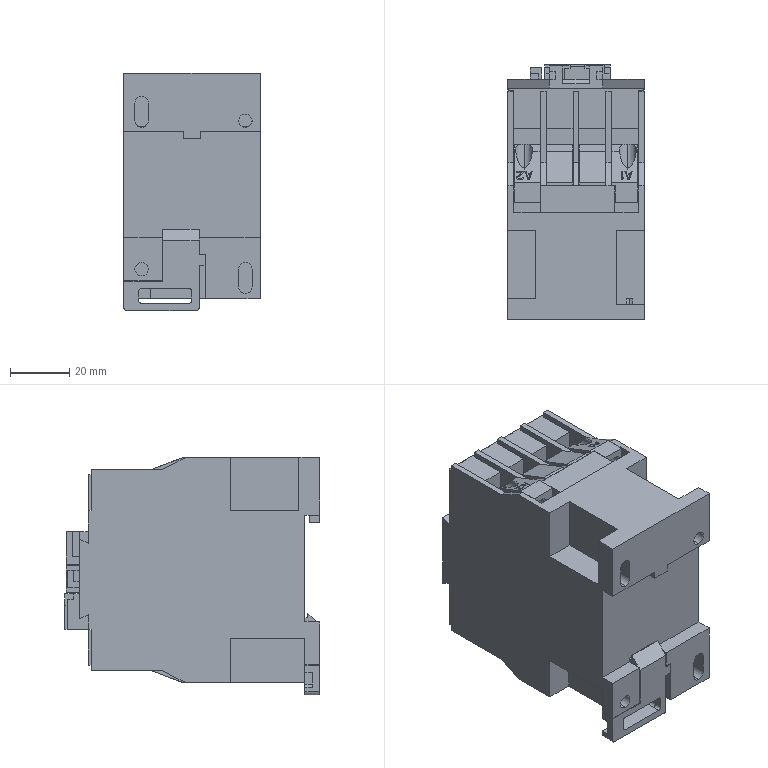Part | STEP file | cjx2_d18.step | 1 solid | 1365 faces | box 46 x 86.1 x 80 mm | volume 227917 mm3 | plane 1326 | cylinder 39 | commonest cylinder face diameters 7 x12 4.5 x10 6 x10 2 x7